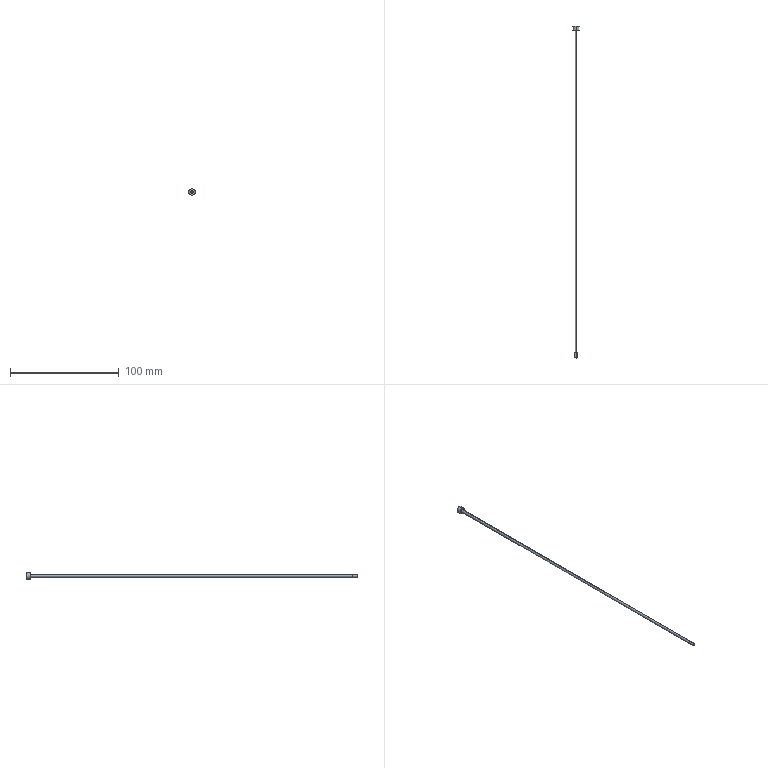Part | STEP file | 1 solid | 9 faces | box 6 x 304.798 x 6 mm | volume 1589 mm3 | cylinder 4 | plane 3 | cone 2 | commonest cylinder face diameters 2.5 x2 6 x2
STEP:
#1=CARTESIAN_POINT('',(0.,0.,0.));
#2=DIRECTION('',(0.,0.,1.));
#3=DIRECTION('',(1.,0.,0.));
#4=AXIS2_PLACEMENT_3D('',#1,#2,#3);
#5=CARTESIAN_POINT('',(-37.688,345.5,103.53));
#6=VERTEX_POINT('',#5);
#7=CARTESIAN_POINT('',(-37.688,345.5,109.53));
#8=VERTEX_POINT('',#7);
#9=CARTESIAN_POINT('',(-37.688,345.5,106.53));
#10=DIRECTION('',(0.,-1.,0.));
#11=DIRECTION('',(0.,0.,-1.));
#12=AXIS2_PLACEMENT_3D('',#9,#10,#11);
#13=CIRCLE('',#12,3.);
#14=CARTESIAN_POINT('',(-37.688,345.5,106.53));
#15=DIRECTION('',(0.,-1.,0.));
#16=DIRECTION('',(0.,0.,-1.));
#17=AXIS2_PLACEMENT_3D('',#14,#15,#16);
#18=CYLINDRICAL_SURFACE('',#17,3.);
#19=CARTESIAN_POINT('',(0.,0.));
#20=DIRECTION('',(1.,0.));
#21=VECTOR('',#20,1.);
#22=LINE('',#19,#21);
#23=(GEOMETRIC_REPRESENTATION_CONTEXT(2)PARAMETRIC_REPRESENTATION_CONTEXT()REPRESENTATION_CONTEXT('',''));
#24=DEFINITIONAL_REPRESENTATION('',(#22),#23);
#25=PCURVE('',#18,#24);
#26=CARTESIAN_POINT('',(-72.862,345.5,110.196));
#27=DIRECTION('',(0.,-1.,0.));
#28=DIRECTION('',(0.,0.,-1.));
#29=AXIS2_PLACEMENT_3D('',#26,#27,#28);
#30=PLANE('',#29);
#31=CARTESIAN_POINT('',(3.666,35.175));
#32=DIRECTION('',(1.,0.));
#33=AXIS2_PLACEMENT_2D('',#31,#32);
#34=CIRCLE('',#33,3.);
#35=(GEOMETRIC_REPRESENTATION_CONTEXT(2)PARAMETRIC_REPRESENTATION_CONTEXT()REPRESENTATION_CONTEXT('',''));
#36=DEFINITIONAL_REPRESENTATION('',(#34),#35);
#37=PCURVE('',#30,#36);
#38=SURFACE_CURVE('',#13,(#25,#37),.PCURVE_S1.);
#39=EDGE_CURVE('',#6,#8,#38,.T.);
#40=ORIENTED_EDGE('',*,*,#39,.T.);
#41=CARTESIAN_POINT('',(-37.688,341.5,109.53));
#42=VERTEX_POINT('',#41);
#43=CARTESIAN_POINT('',(-37.688,345.5,109.53));
#44=DIRECTION('',(0.,-1.,0.));
#45=VECTOR('',#44,1.);
#46=LINE('',#43,#45);
#47=CARTESIAN_POINT('',(3.142,0.));
#48=DIRECTION('',(0.,1.));
#49=VECTOR('',#48,1.);
#50=LINE('',#47,#49);
#51=(GEOMETRIC_REPRESENTATION_CONTEXT(2)PARAMETRIC_REPRESENTATION_CONTEXT()REPRESENTATION_CONTEXT('',''));
#52=DEFINITIONAL_REPRESENTATION('',(#50),#51);
#53=PCURVE('',#18,#52);
#54=CARTESIAN_POINT('',(-37.688,345.5,106.53));
#55=DIRECTION('',(0.,-1.,0.));
#56=DIRECTION('',(0.,0.,-1.));
#57=AXIS2_PLACEMENT_3D('',#54,#55,#56);
#58=CYLINDRICAL_SURFACE('',#57,3.);
#59=CARTESIAN_POINT('',(3.142,0.));
#60=DIRECTION('',(0.,1.));
#61=VECTOR('',#60,1.);
#62=LINE('',#59,#61);
#63=(GEOMETRIC_REPRESENTATION_CONTEXT(2)PARAMETRIC_REPRESENTATION_CONTEXT()REPRESENTATION_CONTEXT('',''));
#64=DEFINITIONAL_REPRESENTATION('',(#62),#63);
#65=PCURVE('',#58,#64);
#66=SURFACE_CURVE('',#46,(#53,#65),.PCURVE_S1.);
#67=EDGE_CURVE('',#8,#42,#66,.T.);
#68=ORIENTED_EDGE('',*,*,#67,.T.);
#69=CARTESIAN_POINT('',(-37.688,341.5,103.53));
#70=VERTEX_POINT('',#69);
#71=CARTESIAN_POINT('',(-37.688,341.5,106.53));
#72=DIRECTION('',(0.,1.,0.));
#73=DIRECTION('',(0.,0.,1.));
#74=AXIS2_PLACEMENT_3D('',#71,#72,#73);
#75=CIRCLE('',#74,3.);
#76=CARTESIAN_POINT('',(3.142,4.));
#77=DIRECTION('',(-1.,0.));
#78=VECTOR('',#77,1.);
#79=LINE('',#76,#78);
#80=(GEOMETRIC_REPRESENTATION_CONTEXT(2)PARAMETRIC_REPRESENTATION_CONTEXT()REPRESENTATION_CONTEXT('',''));
#81=DEFINITIONAL_REPRESENTATION('',(#79),#80);
#82=PCURVE('',#18,#81);
#83=CARTESIAN_POINT('',(-37.688,341.5,106.53));
#84=DIRECTION('',(0.,-1.,0.));
#85=DIRECTION('',(0.,0.,-1.));
#86=AXIS2_PLACEMENT_3D('',#83,#84,#85);
#87=PLANE('',#86);
#88=CARTESIAN_POINT('',(-3.,0.));
#89=CARTESIAN_POINT('',(-3.,5.196));
#90=CARTESIAN_POINT('',(1.5,2.598));
#91=CARTESIAN_POINT('',(6.,0.));
#92=CARTESIAN_POINT('',(1.5,-2.598));
#93=CARTESIAN_POINT('',(-3.,-5.196));
#94=CARTESIAN_POINT('',(-3.,0.));
#95=(BOUNDED_CURVE()B_SPLINE_CURVE(2,(#88,#89,#90,#91,#92,#93,#94),.UNSPECIFIED.,.T.,.F.)B_SPLINE_CURVE_WITH_KNOTS((1,2,2,2,2,1),(-2.094,0.,2.094,4.189,6.283,8.378),.UNSPECIFIED.)CURVE()GEOMETRIC_REPRESENTATION_ITEM()RATIONAL_B_SPLINE_CURVE((1.,0.5,1.,0.5,1.,0.5,1.))REPRESENTATION_ITEM(''));
#96=(GEOMETRIC_REPRESENTATION_CONTEXT(2)PARAMETRIC_REPRESENTATION_CONTEXT()REPRESENTATION_CONTEXT('',''));
#97=DEFINITIONAL_REPRESENTATION('',(#95),#96);
#98=PCURVE('',#87,#97);
#99=SURFACE_CURVE('',#75,(#82,#98),.PCURVE_S1.);
#100=EDGE_CURVE('',#42,#70,#99,.T.);
#101=ORIENTED_EDGE('',*,*,#100,.T.);
#102=CARTESIAN_POINT('',(-37.688,345.5,103.53));
#103=DIRECTION('',(0.,-1.,0.));
#104=VECTOR('',#103,1.);
#105=LINE('',#102,#104);
#106=CARTESIAN_POINT('',(0.,0.));
#107=DIRECTION('',(0.,1.));
#108=VECTOR('',#107,1.);
#109=LINE('',#106,#108);
#110=(GEOMETRIC_REPRESENTATION_CONTEXT(2)PARAMETRIC_REPRESENTATION_CONTEXT()REPRESENTATION_CONTEXT('',''));
#111=DEFINITIONAL_REPRESENTATION('',(#109),#110);
#112=PCURVE('',#18,#111);
#113=CARTESIAN_POINT('',(6.283,0.));
#114=DIRECTION('',(0.,1.));
#115=VECTOR('',#114,1.);
#116=LINE('',#113,#115);
#117=(GEOMETRIC_REPRESENTATION_CONTEXT(2)PARAMETRIC_REPRESENTATION_CONTEXT()REPRESENTATION_CONTEXT('',''));
#118=DEFINITIONAL_REPRESENTATION('',(#116),#117);
#119=PCURVE('',#58,#118);
#120=SURFACE_CURVE('',#105,(#112,#119),.PCURVE_S1.);
#121=EDGE_CURVE('',#6,#70,#120,.T.);
#122=ORIENTED_EDGE('',*,*,#121,.F.);
#123=EDGE_LOOP('',(#40,#68,#101,#122));
#124=FACE_BOUND('',#123,.T.);
#125=ADVANCED_FACE('',(#124),#18,.T.);
#126=CARTESIAN_POINT('',(-37.688,40.703,105.322));
#127=VERTEX_POINT('',#126);
#128=CARTESIAN_POINT('',(-37.688,40.703,107.738));
#129=VERTEX_POINT('',#128);
#130=CARTESIAN_POINT('',(-37.688,40.703,106.53));
#131=DIRECTION('',(0.,-1.,0.));
#132=DIRECTION('',(0.,0.,1.));
#133=AXIS2_PLACEMENT_3D('',#130,#131,#132);
#134=CIRCLE('',#133,1.208);
#135=CARTESIAN_POINT('',(-37.688,46.23,106.53));
#136=DIRECTION('',(0.,1.,0.));
#137=DIRECTION('',(0.,0.,1.));
#138=AXIS2_PLACEMENT_3D('',#135,#136,#137);
#139=CONICAL_SURFACE('',#138,1.256,0.008727);
#140=CARTESIAN_POINT('',(6.283,-5.527));
#141=DIRECTION('',(-1.,0.));
#142=VECTOR('',#141,1.);
#143=LINE('',#140,#142);
#144=(GEOMETRIC_REPRESENTATION_CONTEXT(2)PARAMETRIC_REPRESENTATION_CONTEXT()REPRESENTATION_CONTEXT('',''));
#145=DEFINITIONAL_REPRESENTATION('',(#143),#144);
#146=PCURVE('',#139,#145);
#147=CARTESIAN_POINT('',(-37.688,40.703,106.53));
#148=DIRECTION('',(0.,-1.,0.));
#149=DIRECTION('',(0.,0.,-1.));
#150=AXIS2_PLACEMENT_3D('',#147,#148,#149);
#151=PLANE('',#150);
#152=CARTESIAN_POINT('',(0.,0.));
#153=DIRECTION('',(-1.,0.));
#154=AXIS2_PLACEMENT_2D('',#152,#153);
#155=CIRCLE('',#154,1.208);
#156=(GEOMETRIC_REPRESENTATION_CONTEXT(2)PARAMETRIC_REPRESENTATION_CONTEXT()REPRESENTATION_CONTEXT('',''));
#157=DEFINITIONAL_REPRESENTATION('',(#155),#156);
#158=PCURVE('',#151,#157);
#159=SURFACE_CURVE('',#134,(#146,#158),.PCURVE_S1.);
#160=EDGE_CURVE('',#127,#129,#159,.T.);
#161=ORIENTED_EDGE('',*,*,#160,.F.);
#162=CARTESIAN_POINT('',(-37.688,45.514,105.28));
#163=VERTEX_POINT('',#162);
#164=CARTESIAN_POINT('',(-37.688,46.23,105.274));
#165=DIRECTION('',(0.,1.,-0.008727));
#166=VECTOR('',#165,1.);
#167=LINE('',#164,#166);
#168=CARTESIAN_POINT('',(3.142,0.));
#169=DIRECTION('',(0.,1.));
#170=VECTOR('',#169,1.);
#171=LINE('',#168,#170);
#172=(GEOMETRIC_REPRESENTATION_CONTEXT(2)PARAMETRIC_REPRESENTATION_CONTEXT()REPRESENTATION_CONTEXT('',''));
#173=DEFINITIONAL_REPRESENTATION('',(#171),#172);
#174=PCURVE('',#139,#173);
#175=CARTESIAN_POINT('',(-37.688,46.23,106.53));
#176=DIRECTION('',(0.,1.,0.));
#177=DIRECTION('',(0.,0.,1.));
#178=AXIS2_PLACEMENT_3D('',#175,#176,#177);
#179=CONICAL_SURFACE('',#178,1.256,0.008727);
#180=CARTESIAN_POINT('',(3.142,0.));
#181=DIRECTION('',(0.,1.));
#182=VECTOR('',#181,1.);
#183=LINE('',#180,#182);
#184=(GEOMETRIC_REPRESENTATION_CONTEXT(2)PARAMETRIC_REPRESENTATION_CONTEXT()REPRESENTATION_CONTEXT('',''));
#185=DEFINITIONAL_REPRESENTATION('',(#183),#184);
#186=PCURVE('',#179,#185);
#187=SURFACE_CURVE('',#167,(#174,#186),.PCURVE_S1.);
#188=EDGE_CURVE('',#127,#163,#187,.T.);
#189=ORIENTED_EDGE('',*,*,#188,.T.);
#190=CARTESIAN_POINT('',(-37.688,45.514,107.78));
#191=VERTEX_POINT('',#190);
#192=CARTESIAN_POINT('',(-37.688,45.514,106.53));
#193=DIRECTION('',(0.,1.,0.));
#194=DIRECTION('',(0.,0.,1.));
#195=AXIS2_PLACEMENT_3D('',#192,#193,#194);
#196=CIRCLE('',#195,1.25);
#197=CARTESIAN_POINT('',(0.,-0.7162));
#198=DIRECTION('',(1.,0.));
#199=VECTOR('',#198,1.);
#200=LINE('',#197,#199);
#201=(GEOMETRIC_REPRESENTATION_CONTEXT(2)PARAMETRIC_REPRESENTATION_CONTEXT()REPRESENTATION_CONTEXT('',''));
#202=DEFINITIONAL_REPRESENTATION('',(#200),#201);
#203=PCURVE('',#139,#202);
#204=CARTESIAN_POINT('',(-37.688,40.703,106.53));
#205=DIRECTION('',(0.,1.,0.));
#206=DIRECTION('',(0.,0.,1.));
#207=AXIS2_PLACEMENT_3D('',#204,#205,#206);
#208=CYLINDRICAL_SURFACE('',#207,1.25);
#209=CARTESIAN_POINT('',(0.,4.811));
#210=DIRECTION('',(1.,0.));
#211=VECTOR('',#210,1.);
#212=LINE('',#209,#211);
#213=(GEOMETRIC_REPRESENTATION_CONTEXT(2)PARAMETRIC_REPRESENTATION_CONTEXT()REPRESENTATION_CONTEXT('',''));
#214=DEFINITIONAL_REPRESENTATION('',(#212),#213);
#215=PCURVE('',#208,#214);
#216=SURFACE_CURVE('',#196,(#203,#215),.PCURVE_S1.);
#217=EDGE_CURVE('',#191,#163,#216,.T.);
#218=ORIENTED_EDGE('',*,*,#217,.F.);
#219=CARTESIAN_POINT('',(-37.688,46.23,107.786));
#220=DIRECTION('',(0.,1.,0.008727));
#221=VECTOR('',#220,1.);
#222=LINE('',#219,#221);
#223=CARTESIAN_POINT('',(0.,0.));
#224=DIRECTION('',(0.,1.));
#225=VECTOR('',#224,1.);
#226=LINE('',#223,#225);
#227=(GEOMETRIC_REPRESENTATION_CONTEXT(2)PARAMETRIC_REPRESENTATION_CONTEXT()REPRESENTATION_CONTEXT('',''));
#228=DEFINITIONAL_REPRESENTATION('',(#226),#227);
#229=PCURVE('',#139,#228);
#230=CARTESIAN_POINT('',(6.283,0.));
#231=DIRECTION('',(0.,1.));
#232=VECTOR('',#231,1.);
#233=LINE('',#230,#232);
#234=(GEOMETRIC_REPRESENTATION_CONTEXT(2)PARAMETRIC_REPRESENTATION_CONTEXT()REPRESENTATION_CONTEXT('',''));
#235=DEFINITIONAL_REPRESENTATION('',(#233),#234);
#236=PCURVE('',#179,#235);
#237=SURFACE_CURVE('',#222,(#229,#236),.PCURVE_S1.);
#238=EDGE_CURVE('',#129,#191,#237,.T.);
#239=ORIENTED_EDGE('',*,*,#238,.F.);
#240=EDGE_LOOP('',(#161,#189,#218,#239));
#241=FACE_BOUND('',#240,.T.);
#242=ADVANCED_FACE('',(#241),#139,.T.);
#243=ORIENTED_EDGE('',*,*,#217,.T.);
#244=CARTESIAN_POINT('',(-37.688,341.5,105.28));
#245=VERTEX_POINT('',#244);
#246=CARTESIAN_POINT('',(-37.688,40.703,105.28));
#247=DIRECTION('',(0.,1.,0.));
#248=VECTOR('',#247,1.);
#249=LINE('',#246,#248);
#250=CARTESIAN_POINT('',(3.142,0.));
#251=DIRECTION('',(0.,1.));
#252=VECTOR('',#251,1.);
#253=LINE('',#250,#252);
#254=(GEOMETRIC_REPRESENTATION_CONTEXT(2)PARAMETRIC_REPRESENTATION_CONTEXT()REPRESENTATION_CONTEXT('',''));
#255=DEFINITIONAL_REPRESENTATION('',(#253),#254);
#256=PCURVE('',#208,#255);
#257=CARTESIAN_POINT('',(-37.688,40.703,106.53));
#258=DIRECTION('',(0.,1.,0.));
#259=DIRECTION('',(0.,0.,1.));
#260=AXIS2_PLACEMENT_3D('',#257,#258,#259);
#261=CYLINDRICAL_SURFACE('',#260,1.25);
#262=CARTESIAN_POINT('',(3.142,0.));
#263=DIRECTION('',(0.,1.));
#264=VECTOR('',#263,1.);
#265=LINE('',#262,#264);
#266=(GEOMETRIC_REPRESENTATION_CONTEXT(2)PARAMETRIC_REPRESENTATION_CONTEXT()REPRESENTATION_CONTEXT('',''));
#267=DEFINITIONAL_REPRESENTATION('',(#265),#266);
#268=PCURVE('',#261,#267);
#269=SURFACE_CURVE('',#249,(#256,#268),.PCURVE_S1.);
#270=EDGE_CURVE('',#163,#245,#269,.T.);
#271=ORIENTED_EDGE('',*,*,#270,.T.);
#272=CARTESIAN_POINT('',(-37.688,341.5,107.78));
#273=VERTEX_POINT('',#272);
#274=CARTESIAN_POINT('',(-37.688,341.5,106.53));
#275=DIRECTION('',(0.,1.,0.));
#276=DIRECTION('',(0.,0.,-1.));
#277=AXIS2_PLACEMENT_3D('',#274,#275,#276);
#278=CIRCLE('',#277,1.25);
#279=CARTESIAN_POINT('',(-3.142,300.798));
#280=DIRECTION('',(1.,0.));
#281=VECTOR('',#280,1.);
#282=LINE('',#279,#281);
#283=(GEOMETRIC_REPRESENTATION_CONTEXT(2)PARAMETRIC_REPRESENTATION_CONTEXT()REPRESENTATION_CONTEXT('',''));
#284=DEFINITIONAL_REPRESENTATION('',(#282),#283);
#285=PCURVE('',#208,#284);
#286=CARTESIAN_POINT('',(1.25,0.));
#287=CARTESIAN_POINT('',(1.25,-2.165));
#288=CARTESIAN_POINT('',(-0.625,-1.083));
#289=CARTESIAN_POINT('',(-2.5,0.));
#290=CARTESIAN_POINT('',(-0.625,1.083));
#291=CARTESIAN_POINT('',(1.25,2.165));
#292=CARTESIAN_POINT('',(1.25,0.));
#293=(BOUNDED_CURVE()B_SPLINE_CURVE(2,(#286,#287,#288,#289,#290,#291,#292),.UNSPECIFIED.,.T.,.F.)B_SPLINE_CURVE_WITH_KNOTS((1,2,2,2,2,1),(-2.094,0.,2.094,4.189,6.283,8.378),.UNSPECIFIED.)CURVE()GEOMETRIC_REPRESENTATION_ITEM()RATIONAL_B_SPLINE_CURVE((1.,0.5,1.,0.5,1.,0.5,1.))REPRESENTATION_ITEM(''));
#294=(GEOMETRIC_REPRESENTATION_CONTEXT(2)PARAMETRIC_REPRESENTATION_CONTEXT()REPRESENTATION_CONTEXT('',''));
#295=DEFINITIONAL_REPRESENTATION('',(#293),#294);
#296=PCURVE('',#87,#295);
#297=SURFACE_CURVE('',#278,(#285,#296),.PCURVE_S1.);
#298=EDGE_CURVE('',#273,#245,#297,.T.);
#299=ORIENTED_EDGE('',*,*,#298,.F.);
#300=CARTESIAN_POINT('',(-37.688,40.703,107.78));
#301=DIRECTION('',(0.,1.,0.));
#302=VECTOR('',#301,1.);
#303=LINE('',#300,#302);
#304=CARTESIAN_POINT('',(0.,0.));
#305=DIRECTION('',(0.,1.));
#306=VECTOR('',#305,1.);
#307=LINE('',#304,#306);
#308=(GEOMETRIC_REPRESENTATION_CONTEXT(2)PARAMETRIC_REPRESENTATION_CONTEXT()REPRESENTATION_CONTEXT('',''));
#309=DEFINITIONAL_REPRESENTATION('',(#307),#308);
#310=PCURVE('',#208,#309);
#311=CARTESIAN_POINT('',(6.283,0.));
#312=DIRECTION('',(0.,1.));
#313=VECTOR('',#312,1.);
#314=LINE('',#311,#313);
#315=(GEOMETRIC_REPRESENTATION_CONTEXT(2)PARAMETRIC_REPRESENTATION_CONTEXT()REPRESENTATION_CONTEXT('',''));
#316=DEFINITIONAL_REPRESENTATION('',(#314),#315);
#317=PCURVE('',#261,#316);
#318=SURFACE_CURVE('',#303,(#310,#317),.PCURVE_S1.);
#319=EDGE_CURVE('',#191,#273,#318,.T.);
#320=ORIENTED_EDGE('',*,*,#319,.F.);
#321=EDGE_LOOP('',(#243,#271,#299,#320));
#322=FACE_BOUND('',#321,.T.);
#323=ADVANCED_FACE('',(#322),#208,.T.);
#324=ORIENTED_EDGE('',*,*,#270,.F.);
#325=CARTESIAN_POINT('',(-37.688,45.514,106.53));
#326=DIRECTION('',(0.,1.,0.));
#327=DIRECTION('',(0.,0.,1.));
#328=AXIS2_PLACEMENT_3D('',#325,#326,#327);
#329=CIRCLE('',#328,1.25);
#330=CARTESIAN_POINT('',(0.,4.811));
#331=DIRECTION('',(1.,0.));
#332=VECTOR('',#331,1.);
#333=LINE('',#330,#332);
#334=(GEOMETRIC_REPRESENTATION_CONTEXT(2)PARAMETRIC_REPRESENTATION_CONTEXT()REPRESENTATION_CONTEXT('',''));
#335=DEFINITIONAL_REPRESENTATION('',(#333),#334);
#336=PCURVE('',#261,#335);
#337=CARTESIAN_POINT('',(0.,-0.7162));
#338=DIRECTION('',(1.,0.));
#339=VECTOR('',#338,1.);
#340=LINE('',#337,#339);
#341=(GEOMETRIC_REPRESENTATION_CONTEXT(2)PARAMETRIC_REPRESENTATION_CONTEXT()REPRESENTATION_CONTEXT('',''));
#342=DEFINITIONAL_REPRESENTATION('',(#340),#341);
#343=PCURVE('',#179,#342);
#344=SURFACE_CURVE('',#329,(#336,#343),.PCURVE_S1.);
#345=EDGE_CURVE('',#163,#191,#344,.T.);
#346=ORIENTED_EDGE('',*,*,#345,.T.);
#347=ORIENTED_EDGE('',*,*,#319,.T.);
#348=CARTESIAN_POINT('',(-37.688,341.5,106.53));
#349=DIRECTION('',(0.,1.,0.));
#350=DIRECTION('',(0.,0.,-1.));
#351=AXIS2_PLACEMENT_3D('',#348,#349,#350);
#352=CIRCLE('',#351,1.25);
#353=CARTESIAN_POINT('',(3.142,300.798));
#354=DIRECTION('',(1.,0.));
#355=VECTOR('',#354,1.);
#356=LINE('',#353,#355);
#357=(GEOMETRIC_REPRESENTATION_CONTEXT(2)PARAMETRIC_REPRESENTATION_CONTEXT()REPRESENTATION_CONTEXT('',''));
#358=DEFINITIONAL_REPRESENTATION('',(#356),#357);
#359=PCURVE('',#261,#358);
#360=CARTESIAN_POINT('',(1.25,0.));
#361=CARTESIAN_POINT('',(1.25,-2.165));
#362=CARTESIAN_POINT('',(-0.625,-1.083));
#363=CARTESIAN_POINT('',(-2.5,0.));
#364=CARTESIAN_POINT('',(-0.625,1.083));
#365=CARTESIAN_POINT('',(1.25,2.165));
#366=CARTESIAN_POINT('',(1.25,0.));
#367=(BOUNDED_CURVE()B_SPLINE_CURVE(2,(#360,#361,#362,#363,#364,#365,#366),.UNSPECIFIED.,.T.,.F.)B_SPLINE_CURVE_WITH_KNOTS((1,2,2,2,2,1),(-2.094,0.,2.094,4.189,6.283,8.378),.UNSPECIFIED.)CURVE()GEOMETRIC_REPRESENTATION_ITEM()RATIONAL_B_SPLINE_CURVE((1.,0.5,1.,0.5,1.,0.5,1.))REPRESENTATION_ITEM(''));
#368=(GEOMETRIC_REPRESENTATION_CONTEXT(2)PARAMETRIC_REPRESENTATION_CONTEXT()REPRESENTATION_CONTEXT('',''));
#369=DEFINITIONAL_REPRESENTATION('',(#367),#368);
#370=PCURVE('',#87,#369);
#371=SURFACE_CURVE('',#352,(#359,#370),.PCURVE_S1.);
#372=EDGE_CURVE('',#245,#273,#371,.T.);
#373=ORIENTED_EDGE('',*,*,#372,.F.);
#374=EDGE_LOOP('',(#324,#346,#347,#373));
#375=FACE_BOUND('',#374,.T.);
#376=ADVANCED_FACE('',(#375),#261,.T.);
#377=ORIENTED_EDGE('',*,*,#188,.F.);
#378=CARTESIAN_POINT('',(-37.688,40.703,106.53));
#379=DIRECTION('',(0.,-1.,0.));
#380=DIRECTION('',(0.,0.,1.));
#381=AXIS2_PLACEMENT_3D('',#378,#379,#380);
#382=CIRCLE('',#381,1.208);
#383=CARTESIAN_POINT('',(6.283,-5.527));
#384=DIRECTION('',(-1.,0.));
#385=VECTOR('',#384,1.);
#386=LINE('',#383,#385);
#387=(GEOMETRIC_REPRESENTATION_CONTEXT(2)PARAMETRIC_REPRESENTATION_CONTEXT()REPRESENTATION_CONTEXT('',''));
#388=DEFINITIONAL_REPRESENTATION('',(#386),#387);
#389=PCURVE('',#179,#388);
#390=CARTESIAN_POINT('',(0.,0.));
#391=DIRECTION('',(-1.,0.));
#392=AXIS2_PLACEMENT_2D('',#390,#391);
#393=CIRCLE('',#392,1.208);
#394=(GEOMETRIC_REPRESENTATION_CONTEXT(2)PARAMETRIC_REPRESENTATION_CONTEXT()REPRESENTATION_CONTEXT('',''));
#395=DEFINITIONAL_REPRESENTATION('',(#393),#394);
#396=PCURVE('',#151,#395);
#397=SURFACE_CURVE('',#382,(#389,#396),.PCURVE_S1.);
#398=EDGE_CURVE('',#129,#127,#397,.T.);
#399=ORIENTED_EDGE('',*,*,#398,.F.);
#400=ORIENTED_EDGE('',*,*,#238,.T.);
#401=ORIENTED_EDGE('',*,*,#345,.F.);
#402=EDGE_LOOP('',(#377,#399,#400,#401));
#403=FACE_BOUND('',#402,.T.);
#404=ADVANCED_FACE('',(#403),#179,.T.);
#405=ORIENTED_EDGE('',*,*,#398,.T.);
#406=ORIENTED_EDGE('',*,*,#160,.T.);
#407=EDGE_LOOP('',(#405,#406));
#408=FACE_BOUND('',#407,.T.);
#409=ADVANCED_FACE('',(#408),#151,.T.);
#410=ORIENTED_EDGE('',*,*,#298,.T.);
#411=ORIENTED_EDGE('',*,*,#372,.T.);
#412=EDGE_LOOP('',(#410,#411));
#413=FACE_BOUND('',#412,.T.);
#414=CARTESIAN_POINT('',(-37.688,341.5,106.53));
#415=DIRECTION('',(0.,1.,0.));
#416=DIRECTION('',(0.,0.,1.));
#417=AXIS2_PLACEMENT_3D('',#414,#415,#416);
#418=CIRCLE('',#417,3.);
#419=CARTESIAN_POINT('',(-3.,0.));
#420=CARTESIAN_POINT('',(-3.,5.196));
#421=CARTESIAN_POINT('',(1.5,2.598));
#422=CARTESIAN_POINT('',(6.,0.));
#423=CARTESIAN_POINT('',(1.5,-2.598));
#424=CARTESIAN_POINT('',(-3.,-5.196));
#425=CARTESIAN_POINT('',(-3.,0.));
#426=(BOUNDED_CURVE()B_SPLINE_CURVE(2,(#419,#420,#421,#422,#423,#424,#425),.UNSPECIFIED.,.T.,.F.)B_SPLINE_CURVE_WITH_KNOTS((1,2,2,2,2,1),(-2.094,0.,2.094,4.189,6.283,8.378),.UNSPECIFIED.)CURVE()GEOMETRIC_REPRESENTATION_ITEM()RATIONAL_B_SPLINE_CURVE((1.,0.5,1.,0.5,1.,0.5,1.))REPRESENTATION_ITEM(''));
#427=(GEOMETRIC_REPRESENTATION_CONTEXT(2)PARAMETRIC_REPRESENTATION_CONTEXT()REPRESENTATION_CONTEXT('',''));
#428=DEFINITIONAL_REPRESENTATION('',(#426),#427);
#429=PCURVE('',#87,#428);
#430=CARTESIAN_POINT('',(9.425,4.));
#431=DIRECTION('',(-1.,0.));
#432=VECTOR('',#431,1.);
#433=LINE('',#430,#432);
#434=(GEOMETRIC_REPRESENTATION_CONTEXT(2)PARAMETRIC_REPRESENTATION_CONTEXT()REPRESENTATION_CONTEXT('',''));
#435=DEFINITIONAL_REPRESENTATION('',(#433),#434);
#436=PCURVE('',#58,#435);
#437=SURFACE_CURVE('',#418,(#429,#436),.PCURVE_S1.);
#438=EDGE_CURVE('',#70,#42,#437,.T.);
#439=ORIENTED_EDGE('',*,*,#438,.F.);
#440=ORIENTED_EDGE('',*,*,#100,.F.);
#441=EDGE_LOOP('',(#439,#440));
#442=FACE_BOUND('',#441,.T.);
#443=ADVANCED_FACE('',(#413,#442),#87,.T.);
#444=ORIENTED_EDGE('',*,*,#67,.F.);
#445=CARTESIAN_POINT('',(-37.688,345.5,106.53));
#446=DIRECTION('',(0.,-1.,0.));
#447=DIRECTION('',(0.,0.,-1.));
#448=AXIS2_PLACEMENT_3D('',#445,#446,#447);
#449=CIRCLE('',#448,3.);
#450=CARTESIAN_POINT('',(0.,0.));
#451=DIRECTION('',(1.,0.));
#452=VECTOR('',#451,1.);
#453=LINE('',#450,#452);
#454=(GEOMETRIC_REPRESENTATION_CONTEXT(2)PARAMETRIC_REPRESENTATION_CONTEXT()REPRESENTATION_CONTEXT('',''));
#455=DEFINITIONAL_REPRESENTATION('',(#453),#454);
#456=PCURVE('',#58,#455);
#457=CARTESIAN_POINT('',(3.666,35.175));
#458=DIRECTION('',(1.,0.));
#459=AXIS2_PLACEMENT_2D('',#457,#458);
#460=CIRCLE('',#459,3.);
#461=(GEOMETRIC_REPRESENTATION_CONTEXT(2)PARAMETRIC_REPRESENTATION_CONTEXT()REPRESENTATION_CONTEXT('',''));
#462=DEFINITIONAL_REPRESENTATION('',(#460),#461);
#463=PCURVE('',#30,#462);
#464=SURFACE_CURVE('',#449,(#456,#463),.PCURVE_S1.);
#465=EDGE_CURVE('',#8,#6,#464,.T.);
#466=ORIENTED_EDGE('',*,*,#465,.T.);
#467=ORIENTED_EDGE('',*,*,#121,.T.);
#468=ORIENTED_EDGE('',*,*,#438,.T.);
#469=EDGE_LOOP('',(#444,#466,#467,#468));
#470=FACE_BOUND('',#469,.T.);
#471=ADVANCED_FACE('',(#470),#58,.T.);
#472=ORIENTED_EDGE('',*,*,#39,.F.);
#473=ORIENTED_EDGE('',*,*,#465,.F.);
#474=EDGE_LOOP('',(#472,#473));
#475=FACE_BOUND('',#474,.T.);
#476=ADVANCED_FACE('',(#475),#30,.F.);
#477=CLOSED_SHELL('',(#125,#242,#323,#376,#404,#409,#443,#471,#476));
#478=MANIFOLD_SOLID_BREP('',#477);
#479=(LENGTH_UNIT()NAMED_UNIT(*)SI_UNIT(.MILLI.,.METRE.));
#480=UNCERTAINTY_MEASURE_WITH_UNIT(LENGTH_MEASURE(0.0000001),#479,'','');
#481=(NAMED_UNIT(*)PLANE_ANGLE_UNIT()SI_UNIT($,.RADIAN.));
#482=(NAMED_UNIT(*)SI_UNIT($,.STERADIAN.)SOLID_ANGLE_UNIT());
#483=(GEOMETRIC_REPRESENTATION_CONTEXT(3)GLOBAL_UNCERTAINTY_ASSIGNED_CONTEXT((#480))GLOBAL_UNIT_ASSIGNED_CONTEXT((#479,#481,#482))REPRESENTATION_CONTEXT('',''));
#484=ADVANCED_BREP_SHAPE_REPRESENTATION('',(#4,#478),#483);